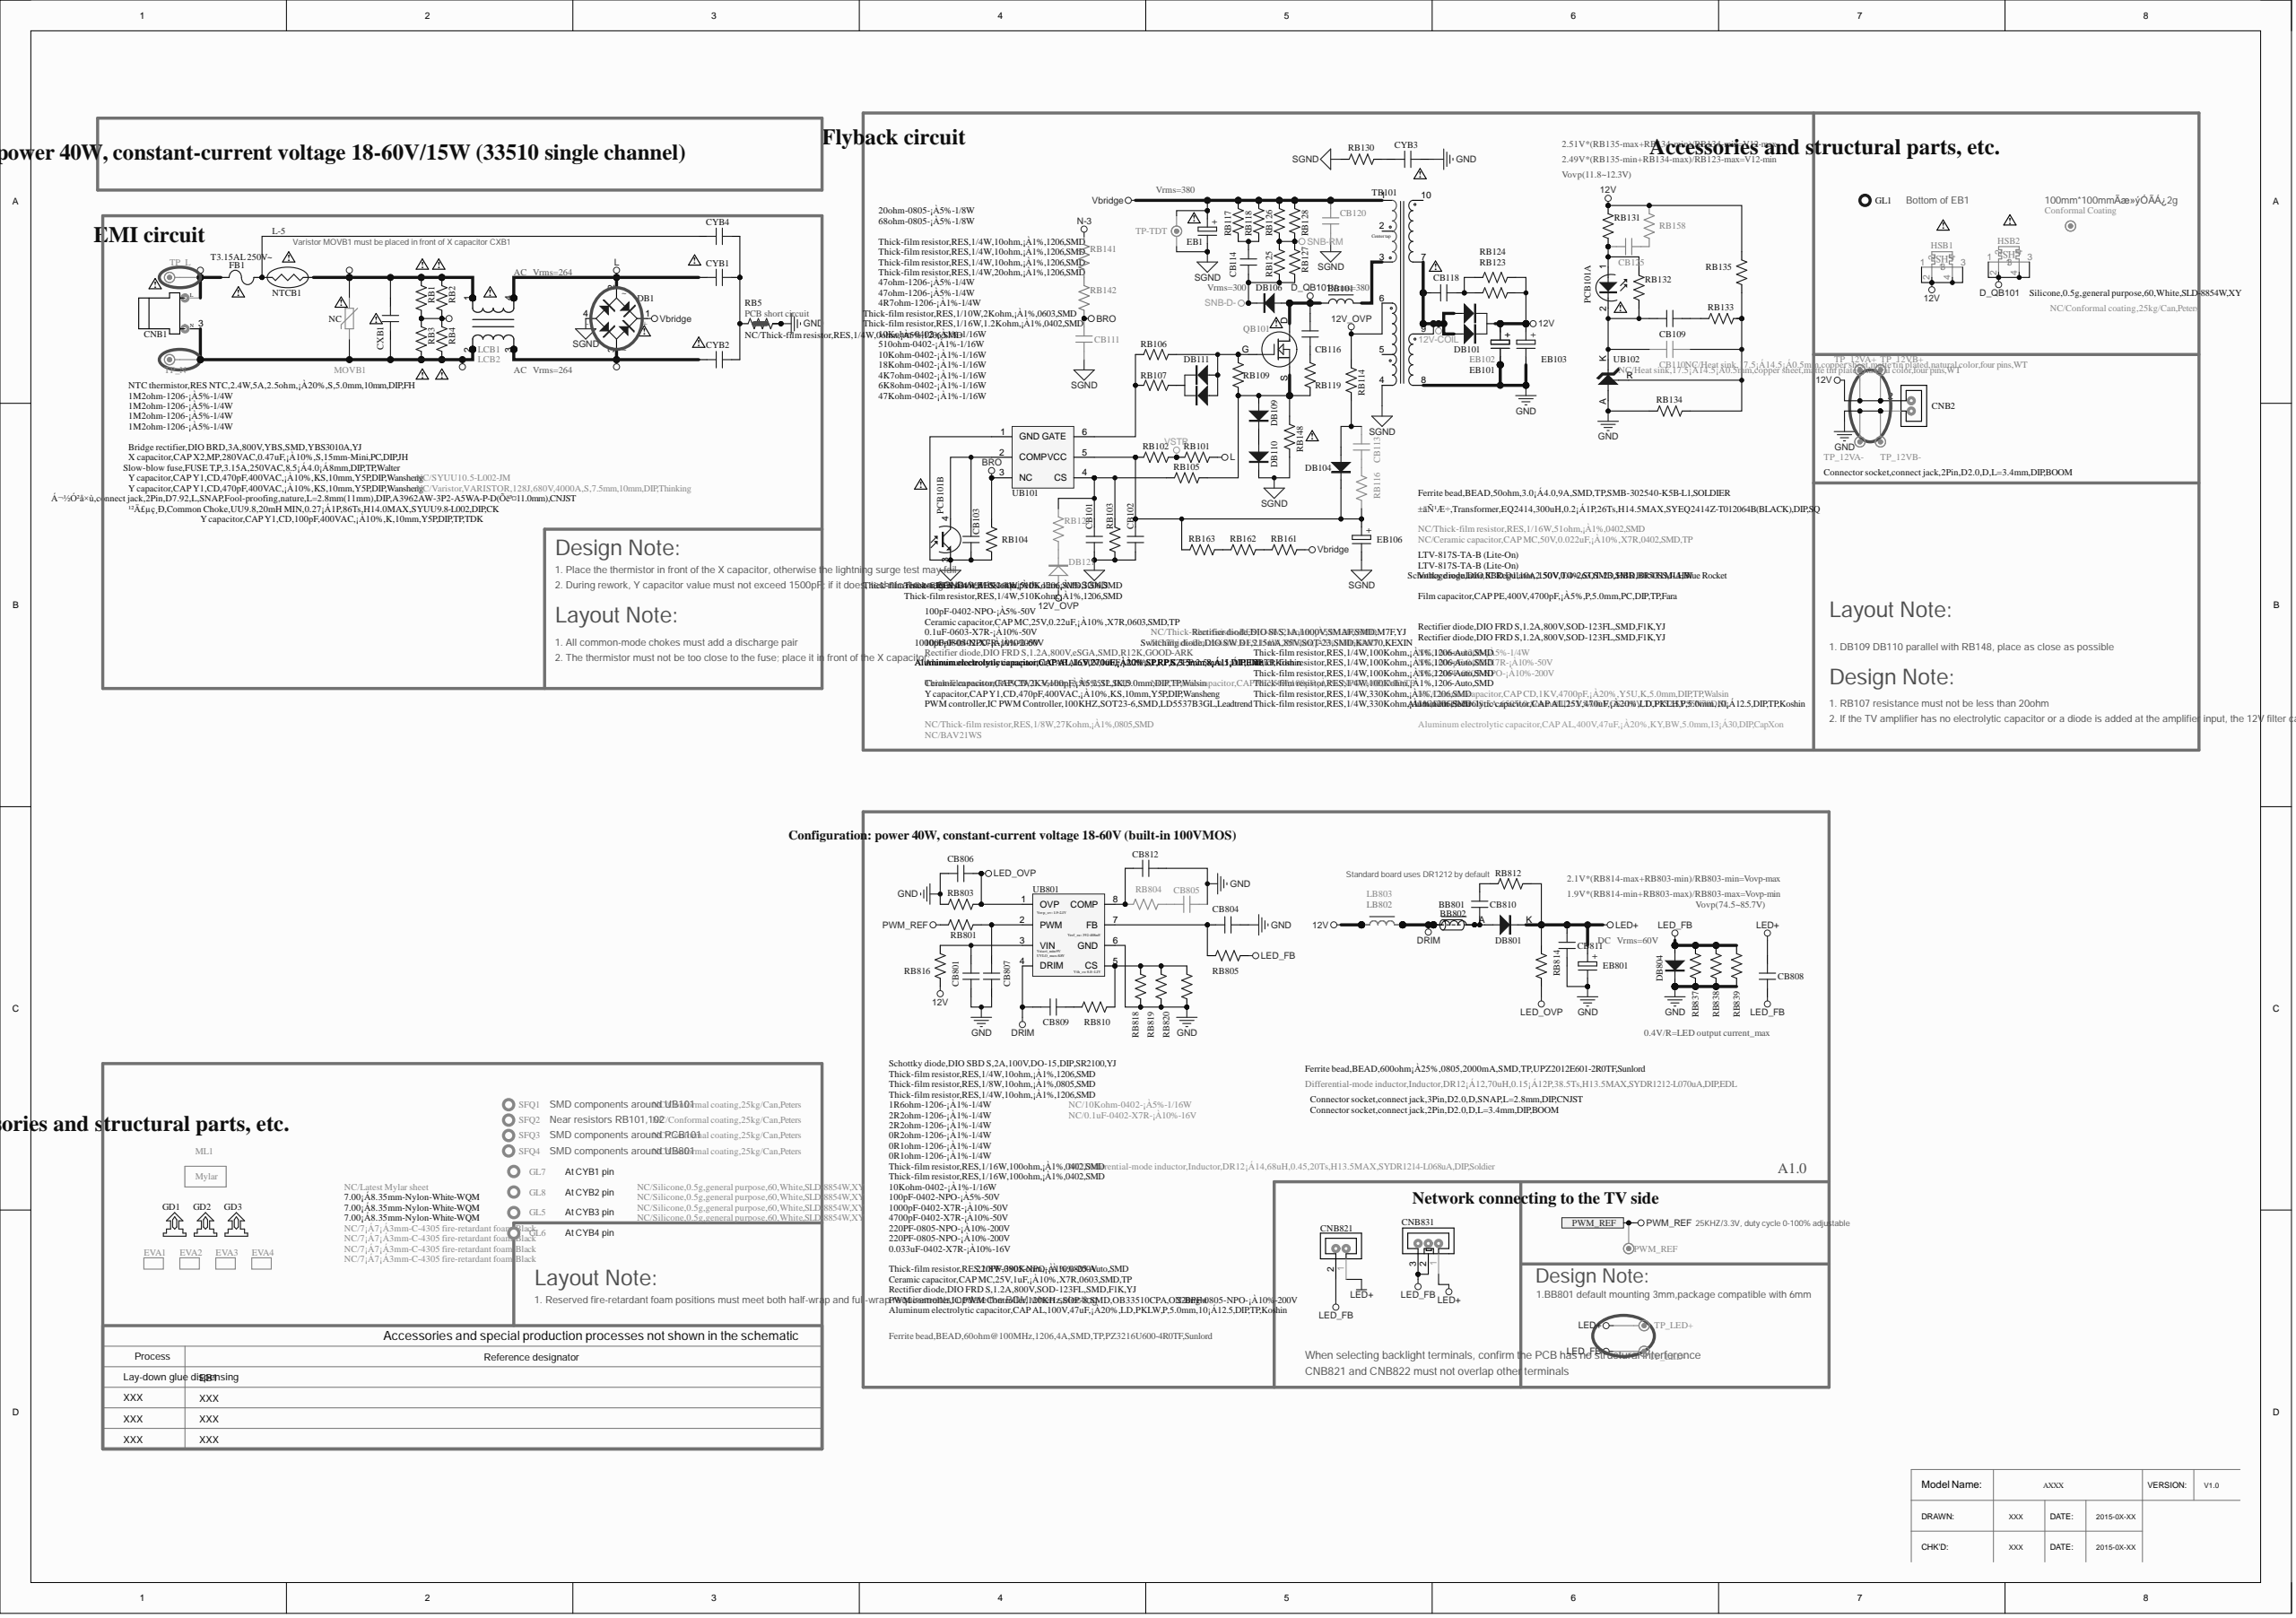Circuit board | Altium Designer | 527 parts | 243 nets | one sheet of the schematic
Parts on this sheet (reference | value | footprint):
BB101 | Ferrite bead,BEAD,50ohm,3.0¡Á4.0,9A,SMD,TP,SMB-302540-K5B-L1,SOLDIER | L(4*3*2.55)-S
BB801 | Ferrite bead,BEAD,60ohm@100MHz,1206,4A,SMD,TP,PZ3216U600-4R0TF,Sunlord | L1206
BB802 | Ferrite bead,BEAD,600ohm¡À25%,0805,2000mA,SMD,TP,UPZ2012E601-2R0TF,Sunlord | L0805
CB101 | 100pF-0402-NPO-¡À5%-50V | C0402
CB102 | 0.1uF-0603-X7R-¡À10%-50V | C0603
CB103 | 1000pF-0402-X7R-¡À10%-50V | C0402
CB109 | Ceramic capacitor,CAP MC,25V,0.22uF,¡À10%,X7R,0603,SMD,TP | C0603
CB110 | NC/1000pF-0402-X7R-¡À10%-50V | C0402
CB111 | NC/Ceramic capacitor,CAP MC,50V,100pF,¡À5%,NPO,0402,SMD,TP | C0402
CB113 | NC/220PF-0805-NPO-¡À10%-200V | C0805
CB114 | Film capacitor,CAP PE,400V,4700pF,¡À5%,P,5.0mm,PC,DIP,TP,Fara | CAP8*2.5-V-5
CB116 | Ceramic capacitor,CAP CD,2KV,100pF,¡À5%,SL,IK,5.0mm,DIP,TP,Walsin | CAP6.5*5-V-5-1
CB118 | 1000pF-0805-NPO-¡À10%-200V | C0805
CB120 | NC/Ceramic capacitor,CAP CD,1KV,4700pF,¡À20%,Y5U,K,5.0mm,DIP,TP,Walsin | CAP10*4.5-V-5
CB125 | NC/Ceramic capacitor,CAP MC,50V,0.022uF,¡À10%,X7R,0402,SMD,TP | C0402
CB801 | Ceramic capacitor,CAP MC,25V,1uF,¡À10%,X7R,0603,SMD,TP | C0603
CB804 | 4700pF-0402-X7R-¡À10%-50V | C0402
CB805 | NC/0.1uF-0402-X7R-¡À10%-16V | C0402
CB806 | 1000pF-0402-X7R-¡À10%-50V | C0402
CB807 | 100pF-0402-NPO-¡À5%-50V | C0402
CB808 | 220PF-0805-NPO-¡À10%-200V | C0805
CB809 | 220PF-0805-NPO-¡À10%-200V | C0805
CB810 | 220PF-0805-NPO-¡À10%-200V | C0805
CB811 | 220PF-0805-NPO-¡À10%-200V | C0805
CB812 | 0.033uF-0402-X7R-¡À10%-16V | C0402
CNB1 | 连接插座,connect jack,2Pin,D7.92,L,SNAP,Fool-proofing,nature,L=2.8mm(11mm),DIP,A3962AW-3P2-A5WA-P-D(针长11.0mm),CNJST | CON2-H7.92
CNB2 | Connector socket,connect jack,2Pin,D2.0,D,L=3.4mm,DIP,BOOM | SIP2/2.0D-1
CNB821 | Connector socket,connect jack,2Pin,D2.0,D,L=3.4mm,DIP,BOOM | SIP2/2.0D-1
CNB831 | Connector socket,connect jack,3Pin,D2.0,D,SNAP,L=2.8mm,DIP,CNJST | SIP3/2.0D-3
CXB1 | X capacitor,CAP X2,MP,280VAC,0.47uF,¡À10%,S,15mm-Mini,PC,DIP,JH | CAP18*8.5-V-15
CYB1 | Y capacitor,CAP Y1,CD,470pF,400VAC,¡À10%,KS,10mm,Y5P,DIP,Wansheng | CAP13*5-V-10-1
CYB2 | Y capacitor,CAP Y1,CD,470pF,400VAC,¡À10%,KS,10mm,Y5P,DIP,Wansheng | CAP13*5-V-10-1
CYB3 | Y capacitor,CAP Y1,CD,470pF,400VAC,¡À10%,KS,10mm,Y5P,DIP,Wansheng | CAP13*5-V-10-1
CYB4 | Y capacitor,CAP Y1,CD,100pF,400VAC,¡À10%,K,10mm,Y5P,DIP,TP,TDK | CAP13*5-V-10-1
DB1 | Bridge rectifier,DIO BRD,3A,800V,YBS,SMD,YBS3010A,YJ | B/YBS3010A
DB101 | Schottky diode,DIO SBD D1,10A,150V,TO-263,SMD,HBR10150SS,JLHW | D2PAK3
DB104 | Rectifier diode,DIO SI S,1A,1000V,SMAF,SMD,M7F,YJ | DIODE-S-1
DB106 | Rectifier diode,DIO FRD S,1.2A,800V,eSGA,SMD,R12K,GOOD-ARK | DIODE-S-14
DB109 | Rectifier diode,DIO FRD S,1.2A,800V,SOD-123FL,SMD,F1K,YJ | DIODE-S-14
DB110 | Rectifier diode,DIO FRD S,1.2A,800V,SOD-123FL,SMD,F1K,YJ | DIODE-S-14
DB111 | Switching diode,DIO SW D1,215mA,85V,SOT-23,SMD,KAV70,KEXIN | SO-23
DB121 | NC/BAV21WS | DIODE-S-12
DB801 | Schottky diode,DIO SBD S,2A,100V,DO-15,DIP,SR2100,YJ | D2-H-15
DB804 | Rectifier diode,DIO FRD S,1.2A,800V,SOD-123FL,SMD,F1K,YJ | DIODE-S-14
EB1 | Aluminum electrolytic capacitor,CAP AL,400V,47uF,¡À20%,KY,BW,5.0mm,13¡Á30,DIP,CapXon | EC(13*30)-H-5
EB101 | Aluminum electrolytic capacitor,CAP AL,16V,270uF,¡À20%,SP,RP,S,3.5mm,8¡Á11,DIP,Elite | EC(8*11)-V-3.5
EB102 | Aluminum electrolytic capacitor,CAP AL,25V,470uF,¡À20%,LD,PKLH,P,5.0mm,10¡Á12.5,DIP,TP,Koshin | EC(10*12.5)-V-5
EB103 | Aluminum electrolytic capacitor,CAP AL,16V,270uF,¡À20%,SP,RP,S,3.5mm,8¡Á11,DIP,Elite | EC(8*11)-V-3.5
EB106 | Aluminum electrolytic capacitor,CAP AL,50V,10uF,¡À20%,LF,PKZF,P,2.5mm,5¡Á11,DIP,TP,Koshin | EC(5*11)-V-2.5
EB801 | Aluminum electrolytic capacitor,CAP AL,100V,47uF,¡À20%,LD,PKLW,P,5.0mm,10¡Á12.5,DIP,TP,Koshin | EC(10*12.5)-V-5
EVA1 | NC/7¡Á7¡Á3mm-C-4305 fire-retardant foam-Black | EVA(7*7*3)
EVA2 | NC/7¡Á7¡Á3mm-C-4305 fire-retardant foam-Black | EVA(7*7*3)
EVA3 | NC/7¡Á7¡Á3mm-C-4305 fire-retardant foam-Black | EVA(7*7*3)
EVA4 | NC/7¡Á7¡Á3mm-C-4305 fire-retardant foam-Black | EVA(7*7*3)
FB1 | Slow-blow fuse,FUSE T,P,3.15A,250VAC,8.5¡Á4.0¡Á8mm,DIP,TP,Walter | FUSE8.5*4-V-5(T3.15AL 250V~)
GD1 | 7.00¡Á8.35mm-Nylon-White-WQM | Fixed
GD2 | 7.00¡Á8.35mm-Nylon-White-WQM | Fixed
GD3 | 7.00¡Á8.35mm-Nylon-White-WQM | Fixed
GL1 | Silicone,0.5g,general purpose,60,White,SLD-8854W,XY | Silica gel-15
GL5 | NC/Silicone,0.5g,general purpose,60,White,SLD-8854W,XY | Silica gel-10
GL6 | NC/Silicone,0.5g,general purpose,60,White,SLD-8854W,XY | Silica gel-10
GL7 | NC/Silicone,0.5g,general purpose,60,White,SLD-8854W,XY | Silica gel-10
GL8 | NC/Silicone,0.5g,general purpose,60,White,SLD-8854W,XY | Silica gel-10
HSB1 | NC/Heat sink,17.5¡Á14.5¡Á0.5mm,copper sheet,matte tin plated,natural color,four pins,WT | HS151-TEMP-NG
HSB2 | NC/Heat sink,17.5¡Á14.5¡Á0.5mm,copper sheet,matte tin plated,natural color,four pins,WT | HS151-TEMP-NG
LB802 | Differential-mode inductor,Inductor,DR12¡Á12,70uH,0.15¡Á12P,38.5Ts,H13.5MAX,SYDR1212-L070uA,DIP,EDL | L/LC2/15*14.5-V7.5
LB803 | NC/Differential-mode inductor,Inductor,DR12¡Á14,68uH,0.45,20Ts,H13.5MAX,SYDR1214-L068uA,DIP,Soldier | L(13.5*15.5)-V-5
LCB1 | 共模电感,Common Choke,UU9.8,20mH MIN,0.27×1P,86Ts,H14.0MAX,SYUU9.8-L002,DIP,CK | L/LC4/UU9.8/7*8-H
LCB2 | NC/SYUU10.5-L002-JM | L/UU10.5/10*13-2
ML1 | NC/Latest Mylar sheet | Mylar
MOVB1 | NC/Varistor,VARISTOR,128J,680V,4000A,S,7.5mm,10mm,DIP,Thinking | VR(13*5)-V-7.5
NTCB1 | NTC thermistor,RES NTC,2.4W,5A,2.5ohm,¡À20%,S,5.0mm,10mm,DIP,FH | NTC(10*5)-V5
PCB101 | LTV-817S-TA-B (Lite-On) | OC4-S-1
QB101 | MOSFET,NMOS,5A,650V,0.8ohm@ID=2.5A@VGS=10V,TO-252,SVS5N70D,SL | TO-252-GDS
RB1 | 1M2ohm-1206-¡À5%-1/4W | R1206
RB2 | 1M2ohm-1206-¡À5%-1/4W | R1206
RB3 | 1M2ohm-1206-¡À5%-1/4W | R1206
RB4 | 1M2ohm-1206-¡À5%-1/4W | R1206
RB5 | NC/Thick-film resistor,RES,1/4W,0ohm,¡À5%,1206,SMD | R1206SC
RB101 | Thick-film resistor,RES,1/4W,330Kohm,¡À1%,1206,SMD | R1206
RB102 | Thick-film resistor,RES,1/4W,330Kohm,¡À1%,1206,SMD | R1206
RB103 | 6K8ohm-0402-¡À1%-1/16W | R0402
RB104 | 47Kohm-0402-¡À1%-1/16W | R0402
RB105 | 510ohm-0402-¡À1%-1/16W | R0402
RB106 | 68ohm-0805-¡À5%-1/8W | R0805
RB107 | 20ohm-0805-¡À5%-1/8W | R0805
RB109 | 10Kohm-0402-¡À1%-1/16W | R0402
RB114 | 4R7ohm-1206-¡À1%-1/4W | R1206
RB116 | NC/10ohm-1206-¡À5%-1/4W | R1206
RB117 | Thick-film resistor,RES,1/4W,10ohm,¡À1%,1206,SMD | R1206
RB118 | Thick-film resistor,RES,1/4W,10ohm,¡À1%,1206,SMD | R1206
RB119 | Thick-film resistor,RES,1/4W,10ohm,¡À1%,1206,SMD | R1206
RB121 | NC/Thick-film resistor,RES,1/8W,27Kohm,¡À1%,0805,SMD | R0805
RB123 | 47ohm-1206-¡À5%-1/4W | R1206
RB124 | 47ohm-1206-¡À5%-1/4W | R1206
RB125 | Thick-film resistor,RES,1/4W,100Kohm,¡À1%,1206-Auto,SMD | R1206
RB126 | Thick-film resistor,RES,1/4W,100Kohm,¡À1%,1206-Auto,SMD | R1206
RB127 | Thick-film resistor,RES,1/4W,100Kohm,¡À1%,1206-Auto,SMD | R1206
RB128 | Thick-film resistor,RES,1/4W,100Kohm,¡À1%,1206-Auto,SMD | R1206
RB130 | Thick-film resistor,RES,1/4W,20ohm,¡À1%,1206,SMD | R1206
RB131 | Thick-film resistor,RES,1/10W,2Kohm,¡À1%,0603,SMD | R0603
RB132 | Thick-film resistor,RES,1/16W,1.2Kohm,¡À1%,0402,SMD | R0402
RB133 | 10Kohm-0402-¡À1%-1/16W | R0402
RB134 | 4K7ohm-0402-¡À1%-1/16W | R0402
RB135 | 18Kohm-0402-¡À1%-1/16W | R0402
RB141 | NC/Thick-film resistor,RES,1/4W,2Mohm,¡À5%,1206,SMD | R1206
RB142 | NC/Thick-film resistor,RES,1/4W,2Mohm,¡À5%,1206,SMD | R1206
RB148 | Thick-film resistor,RES,2W,0.36ohm,¡À5%,2512,SMD | R2512-1
RB158 | NC/Thick-film resistor,RES,1/16W,51ohm,¡À1%,0402,SMD | R0402
RB161 | Thick-film resistor,RES,1/4W,510Kohm,¡À1%,1206,SMD | R1206
RB162 | Thick-film resistor,RES,1/4W,510Kohm,¡À1%,1206,SMD | R1206
RB163 | Thick-film resistor,RES,1/4W,510Kohm,¡À1%,1206,SMD | R1206
RB801 | Thick-film resistor,RES,1/16W,100ohm,¡À1%,0402,SMD | R0402
RB803 | 10Kohm-0402-¡À1%-1/16W | R0402
RB804 | NC/10Kohm-0402-¡À5%-1/16W | R0402
RB805 | Thick-film resistor,RES,1/16W,100ohm,¡À1%,0402,SMD | R0402
RB810 | Thick-film resistor,RES,1/4W,10ohm,¡À1%,1206,SMD | R1206
RB812 | Thick-film resistor,RES,1/4W,10ohm,¡À1%,1206,SMD | R1206
RB814 | Thick-film resistor,RES,1/8W,390Kohm,¡À1%,0805-Auto,SMD | R0805
RB816 | Thick-film resistor,RES,1/8W,10ohm,¡À1%,0805,SMD | R0805
RB818 | 0R2ohm-1206-¡À1%-1/4W | R1206
RB819 | 0R1ohm-1206-¡À1%-1/4W | R1206
RB820 | 0R1ohm-1206-¡À1%-1/4W | R1206
RB837 | 1R6ohm-1206-¡À1%-1/4W | R1206
RB838 | 2R2ohm-1206-¡À1%-1/4W | R1206
RB839 | 2R2ohm-1206-¡À1%-1/4W | R1206
SFQ1 | NC/Conformal coating,25kg/Can,Peters | SFQ
SFQ2 | NC/Conformal coating,25kg/Can,Peters | SFQ
SFQ3 | NC/Conformal coating,25kg/Can,Peters | SFQ
SFQ4 | NC/Conformal coating,25kg/Can,Peters | SFQ
TB101 | 变压器,Transformer,EQ2414,300uH,0.2×1P,26Ts,H14.5MAX,SYEQ2414Z-T012064B(BLACK),DIP,SQ | T/EQ2414*10
TP-TDT | NC/ | TP-TDT
TP_12VA+ | NC/ | TP
TP_L | NC/ | TP-80
TP_N | NC/ | TP-80
UB101 | PWM controller,IC PWM Controller,100KHZ,SOT23-6,SMD,LD5537B3GL,Leadtrend | SOT-26
UB102 | Voltage regulator,IC Regulator,2.50V,0.4%,SOT-23,SMD,BR431M-A,Blue Rocket | SOT-23-RAK
UB801 | PWM controller,IC PWM Controller,120KHz,SOP-8,SMD,OB33510CPA,ON-Bright | SO-8A
Nets of these parts (net: part-pin ...):
VSTR: RB101-2 RB102-1
Vbridge: CB120-2 DB1-1 EB1-1 RB117-2 RB118-2 RB126-2 RB128-2 RB161-1 TB101-1 TP-TDT-1
SNB-RM: RB125-2 RB126-1 RB127-2 RB128-1
SNB-D-: CB114-2 DB106-K RB125-1 RB127-1
SGND: CB101-2 CB102-2 CB103-1 CB111-2 CB120-1 DB1-4 DB110-K EB1-2 EB106-2 PCB101-3 RB103-1 RB104-2 RB130-1 RB148-1 TB101-4 TP-TDT-2 UB101-1
PWM_REF: RB801-1
NetRB810_1: RB810-1 RB818-2 RB819-2 RB820-2 UB801-5
NetRB162_2: RB162-2 RB163-1
NetRB161_2: RB161-2 RB162-1
NetRB141_1: RB141-1 RB142-2
NetRB106_1: RB106-1 RB107-1 UB101-6
NetDB121_K: DB121-K RB121-1
NetDB111_2: DB111-2 RB107-2
NetDB111_1: DB111-1 DB111-3 QB101-G RB106-2 RB109-1
NetDB109_K: DB109-K DB110-A
NetDB109_A: DB109-A QB101-S RB105-2 RB109-2 RB119-1 RB148-2
NetCYB3_1: CYB3-1 RB130-2
NetCYB1_2: CYB1-2 CYB2-2 CYB4-2 RB5-1
NetCB812_1: CB812-1 RB804-1 UB801-8
NetCB810_2: CB810-2 RB812-1
NetCB809_1: CB809-1 RB810-2
NetCB807_2: CB807-2 RB801-2 UB801-2
NetCB805_1: CB805-1 RB804-2
NetCB804_2: CB804-2 RB805-1 UB801-7
NetCB801_1: CB801-1 RB816-2 UB801-3
NetCB125_2: CB125-2 RB158-1
NetCB125_1: CB125-1 PCB101-1 RB131-1 RB132-2
NetCB118_2: CB118-2 RB123-1 RB124-1
NetCB116_1: CB116-1 RB119-2
NetCB114_1: CB114-1 RB117-1 RB118-1
NetCB113_2: CB113-2 RB116-2
NetCB113_1: CB113-1 DB104-A RB114-1
NetCB110_2: CB110-2 RB133-2 RB134-2 RB135-2 UB102-R
NetCB109_2: CB109-2 RB133-1
NetCB109_1: CB109-1 CB110-1 PCB101-2 RB132-1 UB102-K
NetCB103_2: CB103-2 PCB101-4 UB101-2
NetCB102_1: CB102-1 DB104-K EB106-1 RB102-2 RB116-1 RB163-2 UB101-5
NetCB101_1: CB101-1 RB103-2 RB105-1 RB121-2 UB101-4
NetBB801_2: BB801-2 BB802-2 CB810-1 DB801-A
NetBB101_2: BB101-2 TB101-3
N-3: CYB2-1 DB1-3 LCB1-3 LCB2-3 RB141-2
N-2: CNB1-3 CXB1-2 LCB1-2 LCB2-2 MOVB1-2 RB3-2 RB4-2 TP_N-1
LED_OVP: CB806-1 RB803-2 RB814-1 UB801-1
LED_FB: CB808-1 CNB821-2 CNB831-2 CNB831-3 DB804-A RB805-2 RB837-2 RB838-2 RB839-1
LED+: CB808-2 CB811-2 CNB821-1 CNB831-1 DB801-K EB801-1 RB812-2 RB814-2
L-N: RB1-2 RB2-2 RB3-1 RB4-1
L-5: CYB4-1 FB1-2 NTCB1-2
L-2: CXB1-1 LCB1-1 LCB2-1 MOVB1-1 NTCB1-1 RB1-1 RB2-1
L-1: CNB1-1 FB1-1 TP_L-1
L: CYB1-1 DB1-2 LCB1-4 LCB2-4 RB101-1
GND: CB801-2 CB804-1 CB805-2 CB806-2 CB807-1 CB811-1 CB812-2 CNB2-1 CYB3-2 DB804-K EB101-2 EB102-2 EB103-2 EB801-2 RB5-2 RB5-3 RB134-1 RB803-1 RB818-1 RB819-1 RB820-1 RB837-1 RB838-1 RB839-2 TB101-8 UB102-A UB801-6
DRIM: BB801-1 BB802-1 CB809-2 LB802-2 LB803-2 UB801-4
D_QB101: BB101-1 CB116-2 DB106-A HSB2-1 HSB2-2 HSB2-3 HSB2-4 QB101-D
BRO: CB111-1 RB104-1 RB142-1 UB101-3
12V_OVP: DB121-A RB114-2 TB101-6
12V-COIL: CB118-1 DB101-1 DB101-3 TB101-7 TB101-9
12V: CNB2-2 DB101-2 EB101-1 EB102-1 EB103-1 HSB1-1 HSB1-2 HSB1-3 HSB1-4 LB802-1 LB803-1 RB123-2 RB124-2 RB131-2 RB135-1 RB158-2 RB816-1 TP_12VA+-1